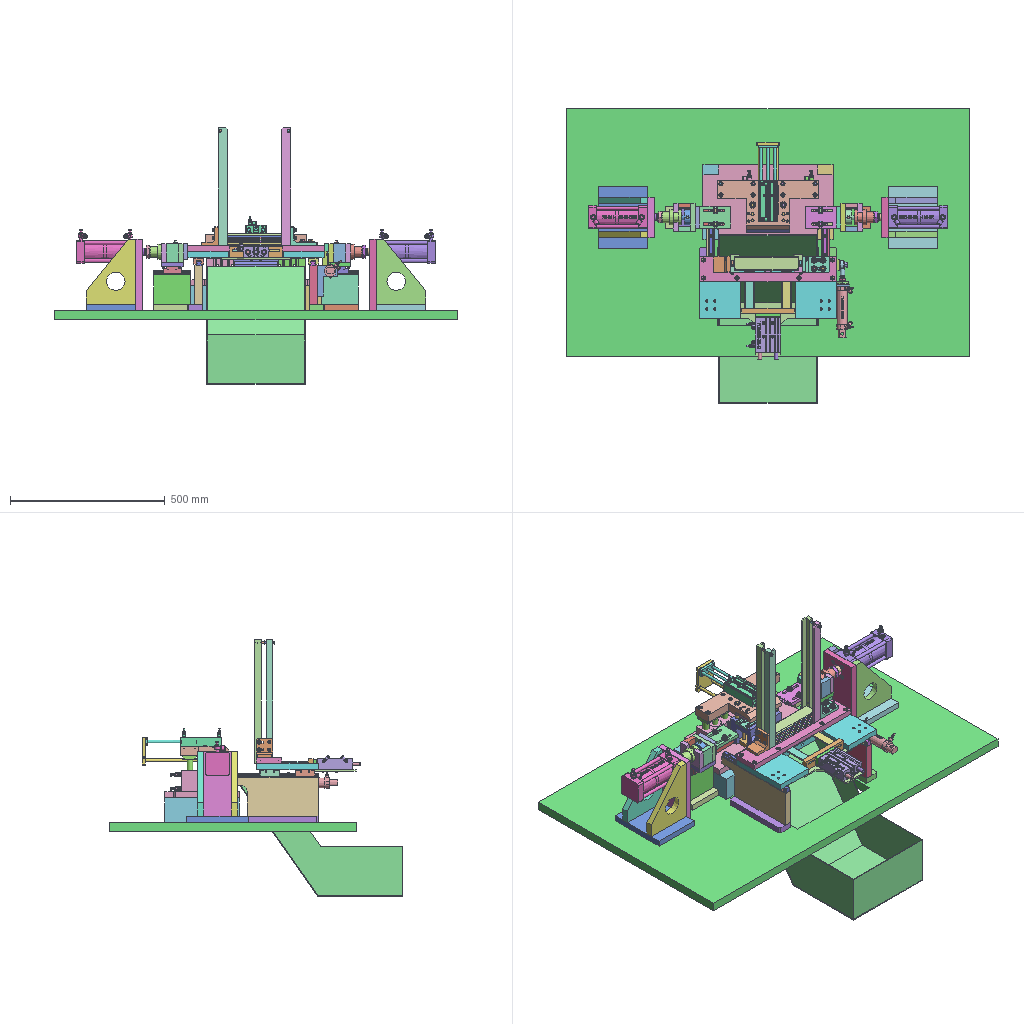Assembly | STEP file | 187 different items | 187 placed | box 1300 x 949 x 829 mm
Parts list (item | name | quantity | size | volume):
1 | Tube necking machine_id750_x_t | x1 | 8.5 x 8.5 x 45 mm | 1022 mm3
2 | Tube necking machine_id746_x_t | x1 | 8.5 x 8.5 x 45 mm | 1022 mm3
3 | Tube necking machine_id742_x_t | x1 | 8.5 x 8.5 x 45 mm | 1022 mm3
4 | Tube necking machine_id738_x_t | x1 | 8.5 x 8.5 x 45 mm | 1022 mm3
5 | Tube necking machine_id734_x_t | x1 | 30 x 134 x 5 mm | 19985 mm3
6 | Tube necking machine_id730_x_t | x1 | 170 x 16 x 35 mm | 90400 mm3
7 | Tube necking machine_id726_x_t | x1 | 111 x 112 x 46.543 mm | 281907 mm3
8 | Tube necking machine_id722_x_t | x1 | 50 x 230 x 20 mm | 229500 mm3
9 | Tube necking machine_id718_x_t | x1 | 25 x 290 x 127 mm | 764196 mm3
10 | Tube necking machine_id714_x_t | x1 | 34 x 61.4 x 23.7 mm | 37642 mm3
11 | Tube necking machine_id710_x_t | x1 | 34 x 61.4 x 23.7 mm | 37642 mm3
12 | Tube necking machine_id706_x_t | x1 | 15 x 290 x 15 mm | 56751 mm3
13 | Tube necking machine_id702_x_t | x1 | 34 x 61.4 x 23.7 mm | 37642 mm3
14 | Tube necking machine_id698_x_t | x1 | 34 x 61.4 x 23.7 mm | 37642 mm3
15 | Tube necking machine_id694_x_t | x1 | 15 x 290 x 15 mm | 56751 mm3
16 | Tube necking machine_id690_x_t | x1 | 220 x 172 x 5 mm | 107264 mm3
17 | Tube necking machine_id686_x_t | x1 | 440 x 82 x 19 mm | 401344 mm3
18 | Tube necking machine_id682_x_t | x1 | 440 x 200 x 20 mm | 1280618 mm3
19 | Tube necking machine_id678_x_t | x1 | 25 x 290 x 127 mm | 764196 mm3
20 | Tube necking machine_id674_x_t | x1 | 50 x 230 x 20 mm | 229500 mm3
21 | Tube necking machine_id670_x_t | x1 | 1300 x 800 x 30 mm | 28708260 mm3
22 | Tube necking machine_id666_x_t | x1 | 52.931 x 179 x 52.931 mm | 134206 mm3
23 | Tube necking machine_id662_x_t | x1 | 65 x 15 x 100 mm | 36804 mm3
24 | Tube necking machine_id658_x_t | x1 | 15 x 35 x 80 mm | 35904 mm3
25 | Tube necking machine_id654_x_t | x1 | 30 x 20 x 400 mm | 151258 mm3
26 | Tube necking machine_id650_x_t | x1 | 85 x 52 x 60 mm | 60680 mm3
27 | Tube necking machine_id646_x_t | x1 | 55 x 52 x 60 mm | 52164 mm3
28 | Tube necking machine_id642_x_t | x1 | 32 x 16 x 16 mm | 3362 mm3
29 | Tube necking machine_id638_x_t | x1 | 41 x 8.5 x 47.343 mm | 8073 mm3
30 | Tube necking machine_id634_x_t | x1 | 18 x 6 x 20.785 mm | 1113 mm3
31 | Tube necking machine_id630_x_t | x1 | 17 x 56.65 x 28 mm | 13077 mm3
32 | Tube necking machine_id626_x_t | x1 | 30 x 134 x 5 mm | 19985 mm3
33 | Tube necking machine_id622_x_t | x1 | 12 x 36 x 41.569 mm | 8555 mm3
34 | Tube necking machine_id618_x_t | x1 | 29 x 50 x 50 mm | 40860 mm3
35 | Tube necking machine_id614_x_t | x1 | 62 x 48 x 48 mm | 70559 mm3
36 | Tube necking machine_id610_x_t | x1 | 49.238 x 13 x 13 mm | 2846 mm3
37 | Tube necking machine_id606_x_t | x1 | 36 x 13 x 13 mm | 2296 mm3
38 | Tube necking machine_id602_x_t | x1 | 49.238 x 13 x 13 mm | 2846 mm3
39 | Tube necking machine_id598_x_t | x1 | 36 x 13 x 13 mm | 2296 mm3
40 | Tube necking machine_id594_x_t | x1 | 131 x 24 x 24 mm | 57517 mm3
41 | Tube necking machine_id590_x_t | x1 | 192 x 75 x 109.4 mm | 879096 mm3
42 | Tube necking machine_id586_x_t | x1 | 70 x 90 x 15 mm | 89384 mm3
43 | Tube necking machine_id582_x_t | x1 | 40 x 15 x 60 mm | 36000 mm3
44 | Tube necking machine_id578_x_t | x1 | 40 x 15 x 60 mm | 36000 mm3
45 | Tube necking machine_id574_x_t | x1 | 15 x 90 x 60 mm | 81000 mm3
46 | Tube necking machine_id570_x_t | x1 | 15 x 90 x 60 mm | 60931 mm3
47 | Tube necking machine_id566_x_t | x1 | 120 x 25 x 96 mm | 284951 mm3
48 | Tube necking machine_id562_x_t | x1 | 120 x 70 x 20 mm | 168000 mm3
49 | Tube necking machine_id558_x_t | x1 | 160 x 20 x 210 mm | 392701 mm3
50 | Tube necking machine_id554_x_t | x1 | 160 x 20 x 210 mm | 392701 mm3
51 | Tube necking machine_id550_x_t | x1 | 20 x 130 x 230 mm | 565563 mm3
52 | Tube necking machine_id546_x_t | x1 | 160 x 200 x 20 mm | 640000 mm3
53 | Tube necking machine_id542_x_t | x1 | 50 x 240 x 80 mm | 960000 mm3
54 | Tube necking machine_id538_x_t | x1 | 131 x 24 x 24 mm | 57494 mm3
55 | Tube necking machine_id534_x_t | x1 | 11.547 x 10 x 11 mm | 702.875 mm3
56 | Tube necking machine_id530_x_t | x1 | 11.547 x 10 x 11 mm | 702.875 mm3
57 | Tube necking machine_id526_x_t | x1 | 160 x 200 x 20 mm | 640000 mm3
58 | Tube necking machine_id522_x_t | x1 | 120 x 70 x 20 mm | 168000 mm3
59 | Tube necking machine_id518_x_t | x1 | 20 x 130 x 230 mm | 565563 mm3
60 | Tube necking machine_id514_x_t | x1 | 160 x 20 x 210 mm | 392701 mm3
61 | Tube necking machine_id510_x_t | x1 | 120 x 15 x 15 mm | 23510 mm3
62 | Tube necking machine_id506_x_t | x1 | 70 x 90 x 15 mm | 89384 mm3
63 | Tube necking machine_id502_x_t | x1 | 120 x 25 x 96 mm | 284951 mm3
64 | Tube necking machine_id498_x_t | x1 | 12 x 36 x 41.569 mm | 8555 mm3
65 | Tube necking machine_id494_x_t | x1 | 36 x 13 x 13 mm | 2296 mm3
66 | Tube necking machine_id490_x_t | x1 | 160 x 20 x 210 mm | 392701 mm3
67 | Tube necking machine_id486_x_t | x1 | 15 x 90 x 60 mm | 60931 mm3
68 | Tube necking machine_id482_x_t | x1 | 40 x 15 x 60 mm | 36000 mm3
69 | Tube necking machine_id478_x_t | x1 | 40 x 15 x 60 mm | 36000 mm3
70 | Tube necking machine_id474_x_t | x1 | 15 x 70 x 50 mm | 52500 mm3
71 | Tube necking machine_id470_x_t | x1 | 62 x 48 x 48 mm | 70561 mm3
72 | Tube necking machine_id466_x_t | x1 | 192 x 75 x 109.4 mm | 879089 mm3
73 | Tube necking machine_id462_x_t | x1 | 49.238 x 13 x 13 mm | 2846 mm3
74 | Tube necking machine_id458_x_t | x1 | 36 x 13 x 13 mm | 2296 mm3
75 | Tube necking machine_id454_x_t | x1 | 49.238 x 13 x 13 mm | 2846 mm3
76 | Tube necking machine_id450_x_t | x1 | 15 x 90 x 60 mm | 81000 mm3
77 | Tube necking machine_id446_x_t | x1 | 61.4 x 34 x 23.7 mm | 37642 mm3
78 | Tube necking machine_id442_x_t | x1 | 29 x 50 x 50 mm | 40860 mm3
79 | Tube necking machine_id438_x_t | x1 | 80 x 70 x 15 mm | 73671 mm3
80 | Tube necking machine_id434_x_t | x1 | 100 x 70 x 15 mm | 75500 mm3
81 | Tube necking machine_id430_x_t | x1 | 15 x 70 x 50 mm | 52500 mm3
82 | Tube necking machine_id426_x_t | x1 | 120 x 15 x 15 mm | 23510 mm3
83 | Tube necking machine_id422_x_t | x1 | 61.4 x 34 x 23.7 mm | 37642 mm3
84 | Tube necking machine_id418_x_t | x1 | 121 x 89 x 69 mm | 423791 mm3
85 | Tube necking machine_id414_x_t | x1 | 420 x 240 x 20 mm | 1855699 mm3
86 | Tube necking machine_id410_x_t | x1 | 50 x 240 x 80 mm | 960000 mm3
87 | Tube necking machine_id406_x_t | x1 | 75 x 196.3 x 90 mm | 90101 mm3
88 | Tube necking machine_id402_x_t | x1 | 18 x 35 x 10 mm | 5773 mm3
89 | Tube necking machine_id398_x_t | x1 | 100 x 70 x 15 mm | 77231 mm3
90 | Tube necking machine_id394_x_t | x1 | 80 x 70 x 15 mm | 73671 mm3
91 | Tube necking machine_id390_x_t | x1 | 20 x 20 x 1.5 mm | 389.174 mm3
92 | Tube necking machine_id386_x_t | x1 | 13 x 13 x 38 mm | 2397 mm3
93 | Tube necking machine_id382_x_t | x1 | 20 x 20 x 1.5 mm | 389.174 mm3
94 | Tube necking machine_id378_x_t | x1 | 20 x 20 x 1.5 mm | 389.174 mm3
95 | Tube necking machine_id374_x_t | x1 | 13 x 13 x 38 mm | 2397 mm3
96 | Tube necking machine_id370_x_t | x1 | 20 x 20 x 1.5 mm | 389.174 mm3
97 | Tube necking machine_id366_x_t | x1 | 13 x 13 x 38 mm | 2397 mm3
98 | Tube necking machine_id362_x_t | x1 | 20 x 20 x 1.5 mm | 389.174 mm3
99 | Tube necking machine_id358_x_t | x1 | 20 x 20 x 1.5 mm | 389.174 mm3
100 | Tube necking machine_id354_x_t | x1 | 20 x 20 x 1.5 mm | 389.174 mm3
101 | Tube necking machine_id350_x_t | x1 | 13 x 13 x 38 mm | 2397 mm3
102 | Tube necking machine_id346_x_t | x1 | 65 x 133 x 58 mm | 191780 mm3
103 | Tube necking machine_id342_x_t | x1 | 326 x 160 x 30 mm | 867669 mm3
104 | Tube necking machine_id338_x_t | x1 | 140 x 100 x 91 mm | 667813 mm3
105 | Tube necking machine_id334_x_t | x1 | 118 x 44 x 103 mm | 136002 mm3
106 | Tube necking machine_id330_x_t | x1 | 121 x 89 x 69 mm | 423791 mm3
107 | Tube necking machine_id326_x_t | x1 | 118 x 44 x 103 mm | 136002 mm3
108 | Tube necking machine_id322_x_t | x1 | 15 x 15 x 75 mm | 13171 mm3
109 | Tube necking machine_id318_x_t | x1 | 15 x 15 x 75 mm | 13171 mm3
110 | Tube necking machine_id314_x_t | x1 | 317 x 542.25 x 381.672 mm | 881739 mm3
111 | Tube necking machine_id310_x_t | x1 | 205 x 45.1 x 5.7 mm | 9751 mm3
112 | Tube necking machine_id306_x_t | x1 | 13 x 13 x 38 mm | 2397 mm3
113 | Tube necking machine_id302_x_t | x1 | 13 x 13 x 38 mm | 2397 mm3
114 | Tube necking machine_id298_x_t | x1 | 13 x 13 x 38 mm | 2397 mm3
115 | Tube necking machine_id294_x_t | x1 | 13 x 13 x 38 mm | 2397 mm3
116 | Tube necking machine_id290_x_t | x1 | 13 x 13 x 38 mm | 2397 mm3
117 | Tube necking machine_id286_x_t | x1 | 13 x 13 x 38 mm | 2397 mm3
118 | Tube necking machine_id282_x_t | x1 | 13 x 13 x 38 mm | 2397 mm3
119 | Tube necking machine_id278_x_t | x1 | 13 x 13 x 38 mm | 2397 mm3
120 | Tube necking machine_id274_x_t | x1 | 13 x 13 x 38 mm | 2397 mm3
121 | Tube necking machine_id270_x_t | x1 | 13 x 13 x 38 mm | 2397 mm3
122 | Tube necking machine_id266_x_t | x1 | 13 x 13 x 38 mm | 2397 mm3
123 | Tube necking machine_id262_x_t | x1 | 13 x 13 x 43 mm | 2648 mm3
124 | Tube necking machine_id258_x_t | x1 | 13 x 13 x 38 mm | 2397 mm3
125 | Tube necking machine_id254_x_t | x1 | 13 x 13 x 38 mm | 2397 mm3
126 | Tube necking machine_id250_x_t | x1 | 50 x 44 x 37.5 mm | 59062 mm3
127 | Tube necking machine_id246_x_t | x1 | 38 x 13 x 13 mm | 2397 mm3
128 | Tube necking machine_id242_x_t | x1 | 38 x 13 x 13 mm | 2397 mm3
129 | Tube necking machine_id238_x_t | x1 | 130 x 40 x 82.5 mm | 90822 mm3
130 | Tube necking machine_id234_x_t | x1 | 1 x 15 x 15 mm | 175.91 mm3
131 | Tube necking machine_id230_x_t | x1 | 31 x 10 x 10 mm | 1086 mm3
132 | Tube necking machine_id226_x_t | x1 | 26 x 10 x 10 mm | 944.548 mm3
133 | Tube necking machine_id222_x_t | x1 | 26 x 10 x 10 mm | 944.548 mm3
134 | Tube necking machine_id218_x_t | x1 | 1 x 15 x 15 mm | 175.91 mm3
135 | Tube necking machine_id214_x_t | x1 | 31 x 10 x 10 mm | 1086 mm3
136 | Tube necking machine_id210_x_t | x1 | 30 x 20 x 400 mm | 151258 mm3
137 | Tube necking machine_id206_x_t | x1 | 10 x 56 x 10 mm | 1793 mm3
138 | Tube necking machine_id202_x_t | x1 | 10 x 5.7 x 11.547 mm | 357.493 mm3
139 | Tube necking machine_id198_x_t | x1 | 30 x 20 x 400 mm | 151442 mm3
140 | Tube necking machine_id194_x_t | x1 | 10 x 5.7 x 11.547 mm | 357.493 mm3
141 | Tube necking machine_id190_x_t | x1 | 10 x 56 x 10 mm | 1793 mm3
142 | Tube necking machine_id186_x_t | x1 | 1 x 15 x 15 mm | 175.91 mm3
143 | Tube necking machine_id182_x_t | x1 | 1 x 15 x 15 mm | 175.91 mm3
144 | Tube necking machine_id178_x_t | x1 | 31 x 10 x 10 mm | 1086 mm3
145 | Tube necking machine_id174_x_t | x1 | 31 x 10 x 10 mm | 1086 mm3
146 | Tube necking machine_id170_x_t | x1 | 26 x 10 x 10 mm | 944.548 mm3
147 | Tube necking machine_id166_x_t | x1 | 26 x 10 x 10 mm | 944.548 mm3
148 | Tube necking machine_id162_x_t | x1 | 20 x 20 x 1.5 mm | 389.174 mm3
149 | Tube necking machine_id158_x_t | x1 | 20 x 20 x 1.5 mm | 389.174 mm3
150 | Tube necking machine_id154_x_t | x1 | 13 x 13 x 38 mm | 2397 mm3
151 | Tube necking machine_id150_x_t | x1 | 20 x 20 x 1.5 mm | 389.174 mm3
152 | Tube necking machine_id146_x_t | x1 | 20 x 20 x 1.5 mm | 389.174 mm3
153 | Tube necking machine_id142_x_t | x1 | 13 x 13 x 38 mm | 2397 mm3
154 | Tube necking machine_id138_x_t | x1 | 20 x 20 x 1.5 mm | 389.174 mm3
155 | Tube necking machine_id134_x_t | x1 | 20 x 20 x 1.5 mm | 389.174 mm3
156 | Tube necking machine_id130_x_t | x1 | 13 x 13 x 38 mm | 2397 mm3
157 | Tube necking machine_id126_x_t | x1 | 20 x 20 x 1.5 mm | 389.174 mm3
158 | Tube necking machine_id122_x_t | x1 | 20 x 20 x 1.5 mm | 389.174 mm3
159 | Tube necking machine_id118_x_t | x1 | 13 x 13 x 38 mm | 2397 mm3
160 | Tube necking machine_id114_x_t | x1 | 30 x 20 x 400 mm | 151442 mm3
161 | Tube necking machine_id110_x_t | x1 | 7 x 7 x 24 mm | 383.547 mm3
162 | Tube necking machine_id106_x_t | x1 | 7 x 7 x 24 mm | 383.547 mm3
163 | Tube necking machine_id102_x_t | x1 | 7 x 7 x 24 mm | 383.547 mm3
164 | Tube necking machine_id98_x_t | x1 | 7 x 7 x 24 mm | 383.547 mm3
165 | Tube necking machine_id94_x_t | x1 | 7 x 7 x 24 mm | 383.547 mm3
166 | Tube necking machine_id90_x_t | x1 | 7 x 7 x 24 mm | 383.547 mm3
167 | Tube necking machine_id86_x_t | x1 | 7 x 7 x 24 mm | 383.547 mm3
168 | Tube necking machine_id82_x_t | x1 | 7 x 7 x 24 mm | 383.547 mm3
169 | Tube necking machine_id78_x_t | x1 | 140 x 55 x 10 mm | 58090 mm3
170 | Tube necking machine_id74_x_t | x1 | 140 x 55 x 10 mm | 58161 mm3
171 | Tube necking machine_id70_x_t | x1 | 21 x 21 x 20 mm | 3379 mm3
172 | Tube necking machine_id66_x_t | x1 | 21 x 21 x 20 mm | 3379 mm3
173 | Tube necking machine_id62_x_t | x1 | 205 x 45.1 x 5.7 mm | 9751 mm3
174 | Tube necking machine_id58_x_t | x1 | 205 x 45.1 x 5.7 mm | 9751 mm3
175 | Tube necking machine_id54_x_t | x1 | 205 x 45.1 x 5.7 mm | 9751 mm3
176 | Tube necking machine_id50_x_t | x1 | 205 x 45.1 x 5.7 mm | 9751 mm3
177 | Tube necking machine_id46_x_t | x1 | 205 x 45.1 x 5.7 mm | 9751 mm3
178 | Tube necking machine_id42_x_t | x1 | 205 x 45.1 x 5.7 mm | 9751 mm3
179 | Tube necking machine_id38_x_t | x1 | 205 x 45.1 x 5.7 mm | 9751 mm3
180 | Tube necking machine_id34_x_t | x1 | 205 x 45.1 x 5.7 mm | 9751 mm3
181 | Tube necking machine_id30_x_t | x1 | 205 x 45.1 x 5.7 mm | 9751 mm3
182 | Tube necking machine_id26_x_t | x1 | 12 x 12 x 32 mm | 2950 mm3
183 | Tube necking machine_id22_x_t | x1 | 62 x 167.8 x 25 mm | 44767 mm3
184 | Tube necking machine_id18_x_t | x1 | 12 x 158 x 12 mm | 17697 mm3
185 | Tube necking machine_id14_x_t | x1 | 12 x 151.5 x 12 mm | 17126 mm3
186 | Tube necking machine_id10_x_t | x1 | 81 x 76.5 x 30 mm | 30169 mm3
187 | Tube necking machine_id6_x_t | x1 | 12 x 151.5 x 12 mm | 17126 mm3
Placements (level | parent | child | x y z in mm | rotation matrix by rows):
1 | subassembly 2 | Tube necking machine_id750_x_t | 0.0 0.0 0.0 | 1 0 0 0 1 0 0 0 1
1 | subassembly 2 | Tube necking machine_id746_x_t | 0.0 0.0 0.0 | 1 0 0 0 1 0 0 0 1
1 | subassembly 2 | Tube necking machine_id742_x_t | 0.0 0.0 0.0 | 1 0 0 0 1 0 0 0 1
1 | subassembly 2 | Tube necking machine_id738_x_t | 0.0 0.0 0.0 | 1 0 0 0 1 0 0 0 1
1 | subassembly 2 | Tube necking machine_id734_x_t | 0.0 0.0 0.0 | 1 0 0 0 1 0 0 0 1
1 | subassembly 2 | Tube necking machine_id730_x_t | 0.0 0.0 0.0 | 1 0 0 0 1 0 0 0 1
1 | subassembly 2 | Tube necking machine_id726_x_t | 0.0 0.0 0.0 | 1 0 0 0 1 0 0 0 1
1 | subassembly 2 | Tube necking machine_id722_x_t | 0.0 0.0 0.0 | 1 0 0 0 1 0 0 0 1
1 | subassembly 2 | Tube necking machine_id718_x_t | 0.0 0.0 0.0 | 1 0 0 0 1 0 0 0 1
1 | subassembly 2 | Tube necking machine_id714_x_t | 0.0 0.0 0.0 | 1 0 0 0 1 0 0 0 1
1 | subassembly 2 | Tube necking machine_id710_x_t | 0.0 0.0 0.0 | 1 0 0 0 1 0 0 0 1
1 | subassembly 2 | Tube necking machine_id706_x_t | 0.0 0.0 0.0 | 1 0 0 0 1 0 0 0 1
1 | subassembly 2 | Tube necking machine_id702_x_t | 0.0 0.0 0.0 | 1 0 0 0 1 0 0 0 1
1 | subassembly 2 | Tube necking machine_id698_x_t | 0.0 0.0 0.0 | 1 0 0 0 1 0 0 0 1
1 | subassembly 2 | Tube necking machine_id694_x_t | 0.0 0.0 0.0 | 1 0 0 0 1 0 0 0 1
1 | subassembly 2 | Tube necking machine_id690_x_t | 0.0 0.0 0.0 | 1 0 0 0 1 0 0 0 1
1 | subassembly 2 | Tube necking machine_id686_x_t | 0.0 0.0 0.0 | 1 0 0 0 1 0 0 0 1
1 | subassembly 2 | Tube necking machine_id682_x_t | 0.0 0.0 0.0 | 1 0 0 0 1 0 0 0 1
1 | subassembly 2 | Tube necking machine_id678_x_t | 0.0 0.0 0.0 | 1 0 0 0 1 0 0 0 1
1 | subassembly 2 | Tube necking machine_id674_x_t | 0.0 0.0 0.0 | 1 0 0 0 1 0 0 0 1
1 | subassembly 2 | Tube necking machine_id670_x_t | 0.0 0.0 0.0 | 1 0 0 0 1 0 0 0 1
1 | subassembly 2 | Tube necking machine_id666_x_t | 0.0 0.0 0.0 | 1 0 0 0 1 0 0 0 1
1 | subassembly 2 | Tube necking machine_id662_x_t | 0.0 0.0 0.0 | 1 0 0 0 1 0 0 0 1
1 | subassembly 2 | Tube necking machine_id658_x_t | 0.0 0.0 0.0 | 1 0 0 0 1 0 0 0 1
1 | subassembly 2 | Tube necking machine_id654_x_t | 0.0 0.0 0.0 | 1 0 0 0 1 0 0 0 1
1 | subassembly 2 | Tube necking machine_id650_x_t | 0.0 0.0 0.0 | 1 0 0 0 1 0 0 0 1
1 | subassembly 2 | Tube necking machine_id646_x_t | 0.0 0.0 0.0 | 1 0 0 0 1 0 0 0 1
1 | subassembly 2 | Tube necking machine_id642_x_t | 0.0 0.0 0.0 | 1 0 0 0 1 0 0 0 1
1 | subassembly 2 | Tube necking machine_id638_x_t | 0.0 0.0 0.0 | 1 0 0 0 1 0 0 0 1
1 | subassembly 2 | Tube necking machine_id634_x_t | 0.0 0.0 0.0 | 1 0 0 0 1 0 0 0 1
1 | subassembly 2 | Tube necking machine_id630_x_t | 0.0 0.0 0.0 | 1 0 0 0 1 0 0 0 1
1 | subassembly 2 | Tube necking machine_id626_x_t | 0.0 0.0 0.0 | 1 0 0 0 1 0 0 0 1
1 | subassembly 2 | Tube necking machine_id622_x_t | 0.0 0.0 0.0 | 1 0 0 0 1 0 0 0 1
1 | subassembly 2 | Tube necking machine_id618_x_t | 0.0 0.0 0.0 | 1 0 0 0 1 0 0 0 1
1 | subassembly 2 | Tube necking machine_id614_x_t | 0.0 0.0 0.0 | 1 0 0 0 1 0 0 0 1
1 | subassembly 2 | Tube necking machine_id610_x_t | 0.0 0.0 0.0 | 1 0 0 0 1 0 0 0 1
1 | subassembly 2 | Tube necking machine_id606_x_t | 0.0 0.0 0.0 | 1 0 0 0 1 0 0 0 1
1 | subassembly 2 | Tube necking machine_id602_x_t | 0.0 0.0 0.0 | 1 0 0 0 1 0 0 0 1
1 | subassembly 2 | Tube necking machine_id598_x_t | 0.0 0.0 0.0 | 1 0 0 0 1 0 0 0 1
1 | subassembly 2 | Tube necking machine_id594_x_t | 0.0 0.0 0.0 | 1 0 0 0 1 0 0 0 1
1 | subassembly 2 | Tube necking machine_id590_x_t | 0.0 0.0 0.0 | 1 0 0 0 1 0 0 0 1
1 | subassembly 2 | Tube necking machine_id586_x_t | 0.0 0.0 0.0 | 1 0 0 0 1 0 0 0 1
1 | subassembly 2 | Tube necking machine_id582_x_t | 0.0 0.0 0.0 | 1 0 0 0 1 0 0 0 1
1 | subassembly 2 | Tube necking machine_id578_x_t | 0.0 0.0 0.0 | 1 0 0 0 1 0 0 0 1
1 | subassembly 2 | Tube necking machine_id574_x_t | 0.0 0.0 0.0 | 1 0 0 0 1 0 0 0 1
1 | subassembly 2 | Tube necking machine_id570_x_t | 0.0 0.0 0.0 | 1 0 0 0 1 0 0 0 1
1 | subassembly 2 | Tube necking machine_id566_x_t | 0.0 0.0 0.0 | 1 0 0 0 1 0 0 0 1
1 | subassembly 2 | Tube necking machine_id562_x_t | 0.0 0.0 0.0 | 1 0 0 0 1 0 0 0 1
1 | subassembly 2 | Tube necking machine_id558_x_t | 0.0 0.0 0.0 | 1 0 0 0 1 0 0 0 1
1 | subassembly 2 | Tube necking machine_id554_x_t | 0.0 0.0 0.0 | 1 0 0 0 1 0 0 0 1
1 | subassembly 2 | Tube necking machine_id550_x_t | 0.0 0.0 0.0 | 1 0 0 0 1 0 0 0 1
1 | subassembly 2 | Tube necking machine_id546_x_t | 0.0 0.0 0.0 | 1 0 0 0 1 0 0 0 1
1 | subassembly 2 | Tube necking machine_id542_x_t | 0.0 0.0 0.0 | 1 0 0 0 1 0 0 0 1
1 | subassembly 2 | Tube necking machine_id538_x_t | 0.0 0.0 0.0 | 1 0 0 0 1 0 0 0 1
1 | subassembly 2 | Tube necking machine_id534_x_t | 0.0 0.0 0.0 | 1 0 0 0 1 0 0 0 1
1 | subassembly 2 | Tube necking machine_id530_x_t | 0.0 0.0 0.0 | 1 0 0 0 1 0 0 0 1
1 | subassembly 2 | Tube necking machine_id526_x_t | 0.0 0.0 0.0 | 1 0 0 0 1 0 0 0 1
1 | subassembly 2 | Tube necking machine_id522_x_t | 0.0 0.0 0.0 | 1 0 0 0 1 0 0 0 1
1 | subassembly 2 | Tube necking machine_id518_x_t | 0.0 0.0 0.0 | 1 0 0 0 1 0 0 0 1
1 | subassembly 2 | Tube necking machine_id514_x_t | 0.0 0.0 0.0 | 1 0 0 0 1 0 0 0 1
1 | subassembly 2 | Tube necking machine_id510_x_t | 0.0 0.0 0.0 | 1 0 0 0 1 0 0 0 1
1 | subassembly 2 | Tube necking machine_id506_x_t | 0.0 0.0 0.0 | 1 0 0 0 1 0 0 0 1
1 | subassembly 2 | Tube necking machine_id502_x_t | 0.0 0.0 0.0 | 1 0 0 0 1 0 0 0 1
1 | subassembly 2 | Tube necking machine_id498_x_t | 0.0 0.0 0.0 | 1 0 0 0 1 0 0 0 1
1 | subassembly 2 | Tube necking machine_id494_x_t | 0.0 0.0 0.0 | 1 0 0 0 1 0 0 0 1
1 | subassembly 2 | Tube necking machine_id490_x_t | 0.0 0.0 0.0 | 1 0 0 0 1 0 0 0 1
1 | subassembly 2 | Tube necking machine_id486_x_t | 0.0 0.0 0.0 | 1 0 0 0 1 0 0 0 1
1 | subassembly 2 | Tube necking machine_id482_x_t | 0.0 0.0 0.0 | 1 0 0 0 1 0 0 0 1
1 | subassembly 2 | Tube necking machine_id478_x_t | 0.0 0.0 0.0 | 1 0 0 0 1 0 0 0 1
1 | subassembly 2 | Tube necking machine_id474_x_t | 0.0 0.0 0.0 | 1 0 0 0 1 0 0 0 1
1 | subassembly 2 | Tube necking machine_id470_x_t | 0.0 0.0 0.0 | 1 0 0 0 1 0 0 0 1
1 | subassembly 2 | Tube necking machine_id466_x_t | 0.0 0.0 0.0 | 1 0 0 0 1 0 0 0 1
1 | subassembly 2 | Tube necking machine_id462_x_t | 0.0 0.0 0.0 | 1 0 0 0 1 0 0 0 1
1 | subassembly 2 | Tube necking machine_id458_x_t | 0.0 0.0 0.0 | 1 0 0 0 1 0 0 0 1
1 | subassembly 2 | Tube necking machine_id454_x_t | 0.0 0.0 0.0 | 1 0 0 0 1 0 0 0 1
1 | subassembly 2 | Tube necking machine_id450_x_t | 0.0 0.0 0.0 | 1 0 0 0 1 0 0 0 1
1 | subassembly 2 | Tube necking machine_id446_x_t | 0.0 0.0 0.0 | 1 0 0 0 1 0 0 0 1
1 | subassembly 2 | Tube necking machine_id442_x_t | 0.0 0.0 0.0 | 1 0 0 0 1 0 0 0 1
1 | subassembly 2 | Tube necking machine_id438_x_t | 0.0 0.0 0.0 | 1 0 0 0 1 0 0 0 1
1 | subassembly 2 | Tube necking machine_id434_x_t | 0.0 0.0 0.0 | 1 0 0 0 1 0 0 0 1
1 | subassembly 2 | Tube necking machine_id430_x_t | 0.0 0.0 0.0 | 1 0 0 0 1 0 0 0 1
1 | subassembly 2 | Tube necking machine_id426_x_t | 0.0 0.0 0.0 | 1 0 0 0 1 0 0 0 1
1 | subassembly 2 | Tube necking machine_id422_x_t | 0.0 0.0 0.0 | 1 0 0 0 1 0 0 0 1
1 | subassembly 2 | Tube necking machine_id418_x_t | 0.0 0.0 0.0 | 1 0 0 0 1 0 0 0 1
1 | subassembly 2 | Tube necking machine_id414_x_t | 0.0 0.0 0.0 | 1 0 0 0 1 0 0 0 1
1 | subassembly 2 | Tube necking machine_id410_x_t | 0.0 0.0 0.0 | 1 0 0 0 1 0 0 0 1
1 | subassembly 2 | Tube necking machine_id406_x_t | 0.0 0.0 0.0 | 1 0 0 0 1 0 0 0 1
1 | subassembly 2 | Tube necking machine_id402_x_t | 0.0 0.0 0.0 | 1 0 0 0 1 0 0 0 1
1 | subassembly 2 | Tube necking machine_id398_x_t | 0.0 0.0 0.0 | 1 0 0 0 1 0 0 0 1
1 | subassembly 2 | Tube necking machine_id394_x_t | 0.0 0.0 0.0 | 1 0 0 0 1 0 0 0 1
1 | subassembly 2 | Tube necking machine_id390_x_t | 0.0 0.0 0.0 | 1 0 0 0 1 0 0 0 1
1 | subassembly 2 | Tube necking machine_id386_x_t | 0.0 0.0 0.0 | 1 0 0 0 1 0 0 0 1
1 | subassembly 2 | Tube necking machine_id382_x_t | 0.0 0.0 0.0 | 1 0 0 0 1 0 0 0 1
1 | subassembly 2 | Tube necking machine_id378_x_t | 0.0 0.0 0.0 | 1 0 0 0 1 0 0 0 1
1 | subassembly 2 | Tube necking machine_id374_x_t | 0.0 0.0 0.0 | 1 0 0 0 1 0 0 0 1
1 | subassembly 2 | Tube necking machine_id370_x_t | 0.0 0.0 0.0 | 1 0 0 0 1 0 0 0 1
1 | subassembly 2 | Tube necking machine_id366_x_t | 0.0 0.0 0.0 | 1 0 0 0 1 0 0 0 1
1 | subassembly 2 | Tube necking machine_id362_x_t | 0.0 0.0 0.0 | 1 0 0 0 1 0 0 0 1
1 | subassembly 2 | Tube necking machine_id358_x_t | 0.0 0.0 0.0 | 1 0 0 0 1 0 0 0 1
1 | subassembly 2 | Tube necking machine_id354_x_t | 0.0 0.0 0.0 | 1 0 0 0 1 0 0 0 1
1 | subassembly 2 | Tube necking machine_id350_x_t | 0.0 0.0 0.0 | 1 0 0 0 1 0 0 0 1
1 | subassembly 2 | Tube necking machine_id346_x_t | 0.0 0.0 0.0 | 1 0 0 0 1 0 0 0 1
1 | subassembly 2 | Tube necking machine_id342_x_t | 0.0 0.0 0.0 | 1 0 0 0 1 0 0 0 1
1 | subassembly 2 | Tube necking machine_id338_x_t | 0.0 0.0 0.0 | 1 0 0 0 1 0 0 0 1
1 | subassembly 2 | Tube necking machine_id334_x_t | 0.0 0.0 0.0 | 1 0 0 0 1 0 0 0 1
1 | subassembly 2 | Tube necking machine_id330_x_t | 0.0 0.0 0.0 | 1 0 0 0 1 0 0 0 1
1 | subassembly 2 | Tube necking machine_id326_x_t | 0.0 0.0 0.0 | 1 0 0 0 1 0 0 0 1
1 | subassembly 2 | Tube necking machine_id322_x_t | 0.0 0.0 0.0 | 1 0 0 0 1 0 0 0 1
1 | subassembly 2 | Tube necking machine_id318_x_t | 0.0 0.0 0.0 | 1 0 0 0 1 0 0 0 1
1 | subassembly 2 | Tube necking machine_id314_x_t | 0.0 0.0 0.0 | 1 0 0 0 1 0 0 0 1
1 | subassembly 2 | Tube necking machine_id310_x_t | 0.0 0.0 0.0 | 1 0 0 0 1 0 0 0 1
1 | subassembly 2 | Tube necking machine_id306_x_t | 0.0 0.0 0.0 | 1 0 0 0 1 0 0 0 1
1 | subassembly 2 | Tube necking machine_id302_x_t | 0.0 0.0 0.0 | 1 0 0 0 1 0 0 0 1
1 | subassembly 2 | Tube necking machine_id298_x_t | 0.0 0.0 0.0 | 1 0 0 0 1 0 0 0 1
1 | subassembly 2 | Tube necking machine_id294_x_t | 0.0 0.0 0.0 | 1 0 0 0 1 0 0 0 1
1 | subassembly 2 | Tube necking machine_id290_x_t | 0.0 0.0 0.0 | 1 0 0 0 1 0 0 0 1
1 | subassembly 2 | Tube necking machine_id286_x_t | 0.0 0.0 0.0 | 1 0 0 0 1 0 0 0 1
1 | subassembly 2 | Tube necking machine_id282_x_t | 0.0 0.0 0.0 | 1 0 0 0 1 0 0 0 1
1 | subassembly 2 | Tube necking machine_id278_x_t | 0.0 0.0 0.0 | 1 0 0 0 1 0 0 0 1
1 | subassembly 2 | Tube necking machine_id274_x_t | 0.0 0.0 0.0 | 1 0 0 0 1 0 0 0 1
1 | subassembly 2 | Tube necking machine_id270_x_t | 0.0 0.0 0.0 | 1 0 0 0 1 0 0 0 1
1 | subassembly 2 | Tube necking machine_id266_x_t | 0.0 0.0 0.0 | 1 0 0 0 1 0 0 0 1
1 | subassembly 2 | Tube necking machine_id262_x_t | 0.0 0.0 0.0 | 1 0 0 0 1 0 0 0 1
1 | subassembly 2 | Tube necking machine_id258_x_t | 0.0 0.0 0.0 | 1 0 0 0 1 0 0 0 1
1 | subassembly 2 | Tube necking machine_id254_x_t | 0.0 0.0 0.0 | 1 0 0 0 1 0 0 0 1
1 | subassembly 2 | Tube necking machine_id250_x_t | 0.0 0.0 0.0 | 1 0 0 0 1 0 0 0 1
1 | subassembly 2 | Tube necking machine_id246_x_t | 0.0 0.0 0.0 | 1 0 0 0 1 0 0 0 1
1 | subassembly 2 | Tube necking machine_id242_x_t | 0.0 0.0 0.0 | 1 0 0 0 1 0 0 0 1
1 | subassembly 2 | Tube necking machine_id238_x_t | 0.0 0.0 0.0 | 1 0 0 0 1 0 0 0 1
1 | subassembly 2 | Tube necking machine_id234_x_t | 0.0 0.0 0.0 | 1 0 0 0 1 0 0 0 1
1 | subassembly 2 | Tube necking machine_id230_x_t | 0.0 0.0 0.0 | 1 0 0 0 1 0 0 0 1
1 | subassembly 2 | Tube necking machine_id226_x_t | 0.0 0.0 0.0 | 1 0 0 0 1 0 0 0 1
1 | subassembly 2 | Tube necking machine_id222_x_t | 0.0 0.0 0.0 | 1 0 0 0 1 0 0 0 1
1 | subassembly 2 | Tube necking machine_id218_x_t | 0.0 0.0 0.0 | 1 0 0 0 1 0 0 0 1
1 | subassembly 2 | Tube necking machine_id214_x_t | 0.0 0.0 0.0 | 1 0 0 0 1 0 0 0 1
1 | subassembly 2 | Tube necking machine_id210_x_t | 0.0 0.0 0.0 | 1 0 0 0 1 0 0 0 1
1 | subassembly 2 | Tube necking machine_id206_x_t | 0.0 0.0 0.0 | 1 0 0 0 1 0 0 0 1
1 | subassembly 2 | Tube necking machine_id202_x_t | 0.0 0.0 0.0 | 1 0 0 0 1 0 0 0 1
1 | subassembly 2 | Tube necking machine_id198_x_t | 0.0 0.0 0.0 | 1 0 0 0 1 0 0 0 1
1 | subassembly 2 | Tube necking machine_id194_x_t | 0.0 0.0 0.0 | 1 0 0 0 1 0 0 0 1
1 | subassembly 2 | Tube necking machine_id190_x_t | 0.0 0.0 0.0 | 1 0 0 0 1 0 0 0 1
1 | subassembly 2 | Tube necking machine_id186_x_t | 0.0 0.0 0.0 | 1 0 0 0 1 0 0 0 1
1 | subassembly 2 | Tube necking machine_id182_x_t | 0.0 0.0 0.0 | 1 0 0 0 1 0 0 0 1
1 | subassembly 2 | Tube necking machine_id178_x_t | 0.0 0.0 0.0 | 1 0 0 0 1 0 0 0 1
1 | subassembly 2 | Tube necking machine_id174_x_t | 0.0 0.0 0.0 | 1 0 0 0 1 0 0 0 1
1 | subassembly 2 | Tube necking machine_id170_x_t | 0.0 0.0 0.0 | 1 0 0 0 1 0 0 0 1
1 | subassembly 2 | Tube necking machine_id166_x_t | 0.0 0.0 0.0 | 1 0 0 0 1 0 0 0 1
1 | subassembly 2 | Tube necking machine_id162_x_t | 0.0 0.0 0.0 | 1 0 0 0 1 0 0 0 1
1 | subassembly 2 | Tube necking machine_id158_x_t | 0.0 0.0 0.0 | 1 0 0 0 1 0 0 0 1
1 | subassembly 2 | Tube necking machine_id154_x_t | 0.0 0.0 0.0 | 1 0 0 0 1 0 0 0 1
1 | subassembly 2 | Tube necking machine_id150_x_t | 0.0 0.0 0.0 | 1 0 0 0 1 0 0 0 1
1 | subassembly 2 | Tube necking machine_id146_x_t | 0.0 0.0 0.0 | 1 0 0 0 1 0 0 0 1
1 | subassembly 2 | Tube necking machine_id142_x_t | 0.0 0.0 0.0 | 1 0 0 0 1 0 0 0 1
1 | subassembly 2 | Tube necking machine_id138_x_t | 0.0 0.0 0.0 | 1 0 0 0 1 0 0 0 1
1 | subassembly 2 | Tube necking machine_id134_x_t | 0.0 0.0 0.0 | 1 0 0 0 1 0 0 0 1
1 | subassembly 2 | Tube necking machine_id130_x_t | 0.0 0.0 0.0 | 1 0 0 0 1 0 0 0 1
1 | subassembly 2 | Tube necking machine_id126_x_t | 0.0 0.0 0.0 | 1 0 0 0 1 0 0 0 1
1 | subassembly 2 | Tube necking machine_id122_x_t | 0.0 0.0 0.0 | 1 0 0 0 1 0 0 0 1
1 | subassembly 2 | Tube necking machine_id118_x_t | 0.0 0.0 0.0 | 1 0 0 0 1 0 0 0 1
1 | subassembly 2 | Tube necking machine_id114_x_t | 0.0 0.0 0.0 | 1 0 0 0 1 0 0 0 1
1 | subassembly 2 | Tube necking machine_id110_x_t | 0.0 0.0 0.0 | 1 0 0 0 1 0 0 0 1
1 | subassembly 2 | Tube necking machine_id106_x_t | 0.0 0.0 0.0 | 1 0 0 0 1 0 0 0 1
1 | subassembly 2 | Tube necking machine_id102_x_t | 0.0 0.0 0.0 | 1 0 0 0 1 0 0 0 1
1 | subassembly 2 | Tube necking machine_id98_x_t | 0.0 0.0 0.0 | 1 0 0 0 1 0 0 0 1
1 | subassembly 2 | Tube necking machine_id94_x_t | 0.0 0.0 0.0 | 1 0 0 0 1 0 0 0 1
1 | subassembly 2 | Tube necking machine_id90_x_t | 0.0 0.0 0.0 | 1 0 0 0 1 0 0 0 1
1 | subassembly 2 | Tube necking machine_id86_x_t | 0.0 0.0 0.0 | 1 0 0 0 1 0 0 0 1
1 | subassembly 2 | Tube necking machine_id82_x_t | 0.0 0.0 0.0 | 1 0 0 0 1 0 0 0 1
1 | subassembly 2 | Tube necking machine_id78_x_t | 0.0 0.0 0.0 | 1 0 0 0 1 0 0 0 1
1 | subassembly 2 | Tube necking machine_id74_x_t | 0.0 0.0 0.0 | 1 0 0 0 1 0 0 0 1
1 | subassembly 2 | Tube necking machine_id70_x_t | 0.0 0.0 0.0 | 1 0 0 0 1 0 0 0 1
1 | subassembly 2 | Tube necking machine_id66_x_t | 0.0 0.0 0.0 | 1 0 0 0 1 0 0 0 1
1 | subassembly 2 | Tube necking machine_id62_x_t | 0.0 0.0 0.0 | 1 0 0 0 1 0 0 0 1
1 | subassembly 2 | Tube necking machine_id58_x_t | 0.0 0.0 0.0 | 1 0 0 0 1 0 0 0 1
1 | subassembly 2 | Tube necking machine_id54_x_t | 0.0 0.0 0.0 | 1 0 0 0 1 0 0 0 1
1 | subassembly 2 | Tube necking machine_id50_x_t | 0.0 0.0 0.0 | 1 0 0 0 1 0 0 0 1
1 | subassembly 2 | Tube necking machine_id46_x_t | 0.0 0.0 0.0 | 1 0 0 0 1 0 0 0 1
1 | subassembly 2 | Tube necking machine_id42_x_t | 0.0 0.0 0.0 | 1 0 0 0 1 0 0 0 1
1 | subassembly 2 | Tube necking machine_id38_x_t | 0.0 0.0 0.0 | 1 0 0 0 1 0 0 0 1
1 | subassembly 2 | Tube necking machine_id34_x_t | 0.0 0.0 0.0 | 1 0 0 0 1 0 0 0 1
1 | subassembly 2 | Tube necking machine_id30_x_t | 0.0 0.0 0.0 | 1 0 0 0 1 0 0 0 1
1 | subassembly 2 | Tube necking machine_id26_x_t | 0.0 0.0 0.0 | 1 0 0 0 1 0 0 0 1
1 | subassembly 2 | Tube necking machine_id22_x_t | 0.0 0.0 0.0 | 1 0 0 0 1 0 0 0 1
1 | subassembly 2 | Tube necking machine_id18_x_t | 0.0 0.0 0.0 | 1 0 0 0 1 0 0 0 1
1 | subassembly 2 | Tube necking machine_id14_x_t | 0.0 0.0 0.0 | 1 0 0 0 1 0 0 0 1
1 | subassembly 2 | Tube necking machine_id10_x_t | 0.0 0.0 0.0 | 1 0 0 0 1 0 0 0 1
1 | subassembly 2 | Tube necking machine_id6_x_t | 0.0 0.0 0.0 | 1 0 0 0 1 0 0 0 1